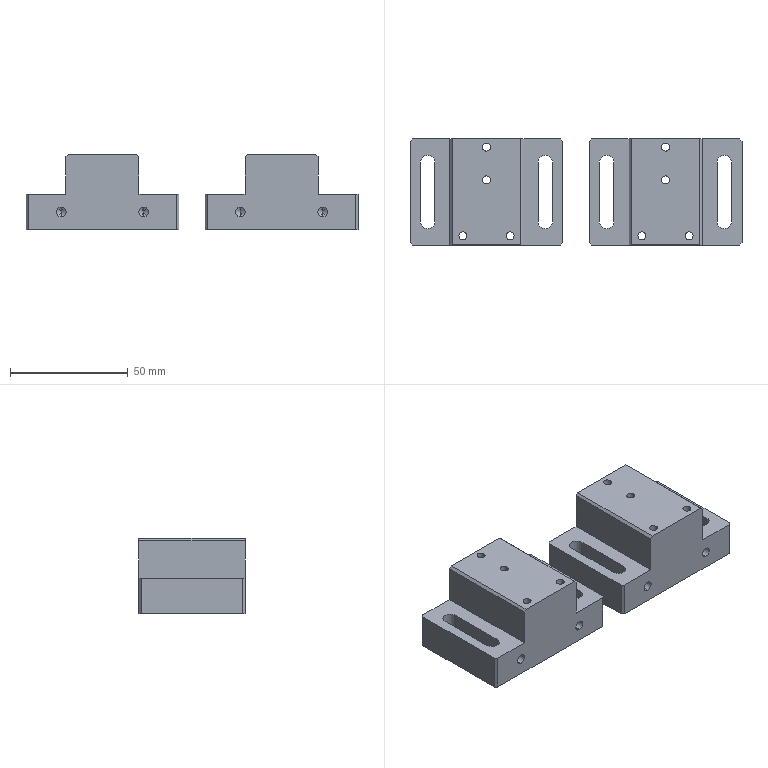NC program | NX | posted with a generic post | part box 140.92 x 45 x 32 mm
Lines 1 to 18 of 6583:
N10 G17 G21 G94 G90
(FLOOR_WALL , TOOL : D80)
N12 T19 M6
N14 G54
N16 G17 G0 G90 X-45. Y22.5 S6500 M3
N18 G43 Z30. H19
N20 Z3.
N22 G94 G1 Z0. F1500.
N24 X-42.
N26 X182.92
N28 X185.92
N30 Z3.
N32 G0 Z30.
N34 M5